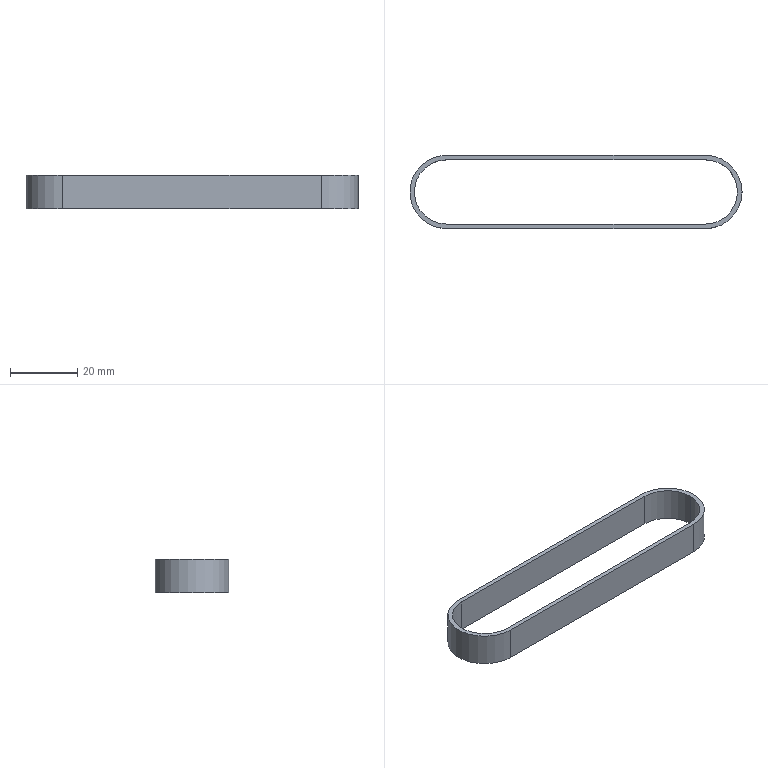Part | SolidWorks | features BaseBody 1 | 1 solid | 12 faces | box 98.817 x 21.817 x 10 mm | volume 2968 mm3 | cylinder 6 | plane 6 | commonest cylinder face diameters 19.097 x3 21.817 x3
STEP:
#1=CARTESIAN_POINT('',(45.526,9.549,0.));
#2=VERTEX_POINT('',#1);
#3=CARTESIAN_POINT('',(55.074,0.,0.));
#4=VERTEX_POINT('',#3);
#5=CARTESIAN_POINT('',(45.526,0.,0.));
#6=DIRECTION('',(0.,0.,-1.));
#7=DIRECTION('',(1.,0.,0.));
#8=AXIS2_PLACEMENT_3D('',#5,#6,#7);
#9=CIRCLE('',#8,9.549);
#10=EDGE_CURVE('',#2,#4,#9,.T.);
#11=ORIENTED_EDGE('',*,*,#10,.T.);
#12=CARTESIAN_POINT('',(55.074,0.,10.));
#13=VERTEX_POINT('',#12);
#14=CARTESIAN_POINT('',(55.074,0.,0.));
#15=DIRECTION('',(0.,0.,1.));
#16=VECTOR('',#15,1000.);
#17=LINE('',#14,#16);
#18=EDGE_CURVE('',#4,#13,#17,.T.);
#19=ORIENTED_EDGE('',*,*,#18,.T.);
#20=CARTESIAN_POINT('',(45.526,9.549,10.));
#21=VERTEX_POINT('',#20);
#22=CARTESIAN_POINT('',(45.526,0.,10.));
#23=DIRECTION('',(0.,0.,-1.));
#24=DIRECTION('',(1.,0.,0.));
#25=AXIS2_PLACEMENT_3D('',#22,#23,#24);
#26=CIRCLE('',#25,9.549);
#27=EDGE_CURVE('',#21,#13,#26,.T.);
#28=ORIENTED_EDGE('',*,*,#27,.F.);
#29=CARTESIAN_POINT('',(45.526,9.549,0.));
#30=DIRECTION('',(0.,0.,-1.));
#31=VECTOR('',#30,1000.);
#32=LINE('',#29,#31);
#33=EDGE_CURVE('',#21,#2,#32,.T.);
#34=ORIENTED_EDGE('',*,*,#33,.T.);
#35=EDGE_LOOP('',(#11,#19,#28,#34));
#36=FACE_OUTER_BOUND('',#35,.T.);
#37=CARTESIAN_POINT('',(45.526,0.,0.));
#38=DIRECTION('',(0.,0.,1.));
#39=DIRECTION('',(1.,0.,0.));
#40=AXIS2_PLACEMENT_3D('',#37,#38,#39);
#41=CYLINDRICAL_SURFACE('',#40,9.549);
#42=ADVANCED_FACE('',(#36),#41,.F.);
#43=CARTESIAN_POINT('',(45.526,-10.908,0.));
#44=VERTEX_POINT('',#43);
#45=CARTESIAN_POINT('',(56.434,0.,0.));
#46=VERTEX_POINT('',#45);
#47=CARTESIAN_POINT('',(45.526,0.,0.));
#48=DIRECTION('',(0.,0.,1.));
#49=DIRECTION('',(1.,0.,0.));
#50=AXIS2_PLACEMENT_3D('',#47,#48,#49);
#51=CIRCLE('',#50,10.909);
#52=EDGE_CURVE('',#44,#46,#51,.T.);
#53=ORIENTED_EDGE('',*,*,#52,.T.);
#54=CARTESIAN_POINT('',(56.434,0.,10.));
#55=VERTEX_POINT('',#54);
#56=CARTESIAN_POINT('',(56.434,0.,0.));
#57=DIRECTION('',(0.,0.,1.));
#58=VECTOR('',#57,1000.);
#59=LINE('',#56,#58);
#60=EDGE_CURVE('',#46,#55,#59,.T.);
#61=ORIENTED_EDGE('',*,*,#60,.T.);
#62=CARTESIAN_POINT('',(45.526,-10.908,10.));
#63=VERTEX_POINT('',#62);
#64=CARTESIAN_POINT('',(45.526,0.,10.));
#65=DIRECTION('',(0.,0.,1.));
#66=DIRECTION('',(1.,0.,0.));
#67=AXIS2_PLACEMENT_3D('',#64,#65,#66);
#68=CIRCLE('',#67,10.909);
#69=EDGE_CURVE('',#63,#55,#68,.T.);
#70=ORIENTED_EDGE('',*,*,#69,.F.);
#71=CARTESIAN_POINT('',(45.526,-10.908,0.));
#72=DIRECTION('',(0.,0.,1.));
#73=VECTOR('',#72,1000.);
#74=LINE('',#71,#73);
#75=EDGE_CURVE('',#44,#63,#74,.T.);
#76=ORIENTED_EDGE('',*,*,#75,.F.);
#77=EDGE_LOOP('',(#53,#61,#70,#76));
#78=FACE_OUTER_BOUND('',#77,.T.);
#79=CARTESIAN_POINT('',(45.526,0.,0.));
#80=DIRECTION('',(0.,0.,1.));
#81=DIRECTION('',(1.,0.,0.));
#82=AXIS2_PLACEMENT_3D('',#79,#80,#81);
#83=CYLINDRICAL_SURFACE('',#82,10.909);
#84=ADVANCED_FACE('',(#78),#83,.T.);
#85=CARTESIAN_POINT('',(-31.474,9.549,0.));
#86=VERTEX_POINT('',#85);
#87=CARTESIAN_POINT('',(-31.474,9.549,10.));
#88=VERTEX_POINT('',#87);
#89=CARTESIAN_POINT('',(-31.474,9.549,0.));
#90=DIRECTION('',(0.,0.,1.));
#91=VECTOR('',#90,1000.);
#92=LINE('',#89,#91);
#93=EDGE_CURVE('',#86,#88,#92,.T.);
#94=ORIENTED_EDGE('',*,*,#93,.F.);
#95=CARTESIAN_POINT('',(-31.474,9.549,0.));
#96=DIRECTION('',(-1.,0.,0.));
#97=VECTOR('',#96,1000.);
#98=LINE('',#95,#97);
#99=EDGE_CURVE('',#2,#86,#98,.T.);
#100=ORIENTED_EDGE('',*,*,#99,.F.);
#101=ORIENTED_EDGE('',*,*,#33,.F.);
#102=CARTESIAN_POINT('',(-31.474,9.549,10.));
#103=DIRECTION('',(1.,0.,0.));
#104=VECTOR('',#103,1000.);
#105=LINE('',#102,#104);
#106=EDGE_CURVE('',#88,#21,#105,.T.);
#107=ORIENTED_EDGE('',*,*,#106,.F.);
#108=EDGE_LOOP('',(#94,#100,#101,#107));
#109=FACE_OUTER_BOUND('',#108,.T.);
#110=CARTESIAN_POINT('',(-31.474,9.549,0.));
#111=DIRECTION('',(0.,1.,0.));
#112=DIRECTION('',(0.,0.,1.));
#113=AXIS2_PLACEMENT_3D('',#110,#111,#112);
#114=PLANE('',#113);
#115=ADVANCED_FACE('',(#109),#114,.F.);
#116=CARTESIAN_POINT('',(45.526,-9.549,10.));
#117=VERTEX_POINT('',#116);
#118=CARTESIAN_POINT('',(-31.474,-9.549,10.));
#119=VERTEX_POINT('',#118);
#120=CARTESIAN_POINT('',(7.026,-9.549,10.));
#121=DIRECTION('',(-1.,0.,0.));
#122=VECTOR('',#121,1000.);
#123=LINE('',#120,#122);
#124=EDGE_CURVE('',#117,#119,#123,.T.);
#125=ORIENTED_EDGE('',*,*,#124,.T.);
#126=CARTESIAN_POINT('',(-31.474,0.,10.));
#127=DIRECTION('',(0.,0.,-1.));
#128=DIRECTION('',(1.,0.,0.));
#129=AXIS2_PLACEMENT_3D('',#126,#127,#128);
#130=CIRCLE('',#129,9.549);
#131=EDGE_CURVE('',#119,#88,#130,.T.);
#132=ORIENTED_EDGE('',*,*,#131,.T.);
#133=ORIENTED_EDGE('',*,*,#106,.T.);
#134=ORIENTED_EDGE('',*,*,#27,.T.);
#135=CARTESIAN_POINT('',(45.526,0.,10.));
#136=DIRECTION('',(0.,0.,-1.));
#137=DIRECTION('',(1.,0.,0.));
#138=AXIS2_PLACEMENT_3D('',#135,#136,#137);
#139=CIRCLE('',#138,9.549);
#140=EDGE_CURVE('',#13,#117,#139,.T.);
#141=ORIENTED_EDGE('',*,*,#140,.T.);
#142=EDGE_LOOP('',(#125,#132,#133,#134,#141));
#143=FACE_BOUND('',#142,.T.);
#144=CARTESIAN_POINT('',(-31.474,10.908,10.));
#145=VERTEX_POINT('',#144);
#146=CARTESIAN_POINT('',(-31.474,-10.908,10.));
#147=VERTEX_POINT('',#146);
#148=CARTESIAN_POINT('',(-31.474,0.,10.));
#149=DIRECTION('',(0.,0.,1.));
#150=DIRECTION('',(1.,0.,0.));
#151=AXIS2_PLACEMENT_3D('',#148,#149,#150);
#152=CIRCLE('',#151,10.909);
#153=EDGE_CURVE('',#145,#147,#152,.T.);
#154=ORIENTED_EDGE('',*,*,#153,.T.);
#155=CARTESIAN_POINT('',(7.026,-10.908,10.));
#156=DIRECTION('',(1.,0.,0.));
#157=VECTOR('',#156,1000.);
#158=LINE('',#155,#157);
#159=EDGE_CURVE('',#147,#63,#158,.T.);
#160=ORIENTED_EDGE('',*,*,#159,.T.);
#161=ORIENTED_EDGE('',*,*,#69,.T.);
#162=CARTESIAN_POINT('',(45.526,10.908,10.));
#163=VERTEX_POINT('',#162);
#164=CARTESIAN_POINT('',(45.526,0.,10.));
#165=DIRECTION('',(0.,0.,1.));
#166=DIRECTION('',(1.,0.,0.));
#167=AXIS2_PLACEMENT_3D('',#164,#165,#166);
#168=CIRCLE('',#167,10.909);
#169=EDGE_CURVE('',#55,#163,#168,.T.);
#170=ORIENTED_EDGE('',*,*,#169,.T.);
#171=CARTESIAN_POINT('',(7.026,10.908,10.));
#172=DIRECTION('',(-1.,0.,0.));
#173=VECTOR('',#172,1000.);
#174=LINE('',#171,#173);
#175=EDGE_CURVE('',#163,#145,#174,.T.);
#176=ORIENTED_EDGE('',*,*,#175,.T.);
#177=EDGE_LOOP('',(#154,#160,#161,#170,#176));
#178=FACE_OUTER_BOUND('',#177,.T.);
#179=CARTESIAN_POINT('',(7.026,0.,10.));
#180=DIRECTION('',(0.,0.,1.));
#181=DIRECTION('',(1.,0.,0.));
#182=AXIS2_PLACEMENT_3D('',#179,#180,#181);
#183=PLANE('',#182);
#184=ADVANCED_FACE('',(#143,#178),#183,.T.);
#185=CARTESIAN_POINT('',(-31.474,-9.549,0.));
#186=VERTEX_POINT('',#185);
#187=CARTESIAN_POINT('',(-31.474,-9.549,0.));
#188=DIRECTION('',(0.,0.,1.));
#189=VECTOR('',#188,1000.);
#190=LINE('',#187,#189);
#191=EDGE_CURVE('',#186,#119,#190,.T.);
#192=ORIENTED_EDGE('',*,*,#191,.F.);
#193=CARTESIAN_POINT('',(-31.474,0.,0.));
#194=DIRECTION('',(0.,0.,1.));
#195=DIRECTION('',(1.,0.,0.));
#196=AXIS2_PLACEMENT_3D('',#193,#194,#195);
#197=CIRCLE('',#196,9.549);
#198=EDGE_CURVE('',#86,#186,#197,.T.);
#199=ORIENTED_EDGE('',*,*,#198,.F.);
#200=ORIENTED_EDGE('',*,*,#93,.T.);
#201=ORIENTED_EDGE('',*,*,#131,.F.);
#202=EDGE_LOOP('',(#192,#199,#200,#201));
#203=FACE_OUTER_BOUND('',#202,.T.);
#204=CARTESIAN_POINT('',(-31.474,0.,0.));
#205=DIRECTION('',(0.,0.,1.));
#206=DIRECTION('',(1.,0.,0.));
#207=AXIS2_PLACEMENT_3D('',#204,#205,#206);
#208=CYLINDRICAL_SURFACE('',#207,9.549);
#209=ADVANCED_FACE('',(#203),#208,.F.);
#210=ORIENTED_EDGE('',*,*,#198,.T.);
#211=CARTESIAN_POINT('',(45.526,-9.549,0.));
#212=VERTEX_POINT('',#211);
#213=CARTESIAN_POINT('',(7.026,-9.549,0.));
#214=DIRECTION('',(-1.,0.,0.));
#215=VECTOR('',#214,1000.);
#216=LINE('',#213,#215);
#217=EDGE_CURVE('',#212,#186,#216,.T.);
#218=ORIENTED_EDGE('',*,*,#217,.F.);
#219=CARTESIAN_POINT('',(45.526,0.,0.));
#220=DIRECTION('',(0.,0.,-1.));
#221=DIRECTION('',(1.,0.,0.));
#222=AXIS2_PLACEMENT_3D('',#219,#220,#221);
#223=CIRCLE('',#222,9.549);
#224=EDGE_CURVE('',#4,#212,#223,.T.);
#225=ORIENTED_EDGE('',*,*,#224,.F.);
#226=ORIENTED_EDGE('',*,*,#10,.F.);
#227=ORIENTED_EDGE('',*,*,#99,.T.);
#228=EDGE_LOOP('',(#210,#218,#225,#226,#227));
#229=FACE_BOUND('',#228,.T.);
#230=ORIENTED_EDGE('',*,*,#52,.F.);
#231=CARTESIAN_POINT('',(-31.474,-10.908,0.));
#232=VERTEX_POINT('',#231);
#233=CARTESIAN_POINT('',(7.026,-10.908,0.));
#234=DIRECTION('',(1.,0.,0.));
#235=VECTOR('',#234,1000.);
#236=LINE('',#233,#235);
#237=EDGE_CURVE('',#232,#44,#236,.T.);
#238=ORIENTED_EDGE('',*,*,#237,.F.);
#239=CARTESIAN_POINT('',(-31.474,10.908,0.));
#240=VERTEX_POINT('',#239);
#241=CARTESIAN_POINT('',(-31.474,0.,0.));
#242=DIRECTION('',(0.,0.,1.));
#243=DIRECTION('',(1.,0.,0.));
#244=AXIS2_PLACEMENT_3D('',#241,#242,#243);
#245=CIRCLE('',#244,10.909);
#246=EDGE_CURVE('',#240,#232,#245,.T.);
#247=ORIENTED_EDGE('',*,*,#246,.F.);
#248=CARTESIAN_POINT('',(45.526,10.908,0.));
#249=VERTEX_POINT('',#248);
#250=CARTESIAN_POINT('',(7.026,10.908,0.));
#251=DIRECTION('',(-1.,0.,0.));
#252=VECTOR('',#251,1000.);
#253=LINE('',#250,#252);
#254=EDGE_CURVE('',#249,#240,#253,.T.);
#255=ORIENTED_EDGE('',*,*,#254,.F.);
#256=CARTESIAN_POINT('',(45.526,0.,0.));
#257=DIRECTION('',(0.,0.,1.));
#258=DIRECTION('',(1.,0.,0.));
#259=AXIS2_PLACEMENT_3D('',#256,#257,#258);
#260=CIRCLE('',#259,10.909);
#261=EDGE_CURVE('',#46,#249,#260,.T.);
#262=ORIENTED_EDGE('',*,*,#261,.F.);
#263=EDGE_LOOP('',(#230,#238,#247,#255,#262));
#264=FACE_OUTER_BOUND('',#263,.T.);
#265=CARTESIAN_POINT('',(7.026,0.,0.));
#266=DIRECTION('',(0.,0.,1.));
#267=DIRECTION('',(1.,0.,0.));
#268=AXIS2_PLACEMENT_3D('',#265,#266,#267);
#269=PLANE('',#268);
#270=ADVANCED_FACE('',(#229,#264),#269,.F.);
#271=ORIENTED_EDGE('',*,*,#18,.F.);
#272=ORIENTED_EDGE('',*,*,#224,.T.);
#273=CARTESIAN_POINT('',(45.526,-9.549,0.));
#274=DIRECTION('',(0.,0.,-1.));
#275=VECTOR('',#274,1000.);
#276=LINE('',#273,#275);
#277=EDGE_CURVE('',#117,#212,#276,.T.);
#278=ORIENTED_EDGE('',*,*,#277,.F.);
#279=ORIENTED_EDGE('',*,*,#140,.F.);
#280=EDGE_LOOP('',(#271,#272,#278,#279));
#281=FACE_OUTER_BOUND('',#280,.T.);
#282=CARTESIAN_POINT('',(45.526,0.,0.));
#283=DIRECTION('',(0.,0.,1.));
#284=DIRECTION('',(1.,0.,0.));
#285=AXIS2_PLACEMENT_3D('',#282,#283,#284);
#286=CYLINDRICAL_SURFACE('',#285,9.549);
#287=ADVANCED_FACE('',(#281),#286,.F.);
#288=ORIENTED_EDGE('',*,*,#277,.T.);
#289=ORIENTED_EDGE('',*,*,#217,.T.);
#290=ORIENTED_EDGE('',*,*,#191,.T.);
#291=ORIENTED_EDGE('',*,*,#124,.F.);
#292=EDGE_LOOP('',(#288,#289,#290,#291));
#293=FACE_OUTER_BOUND('',#292,.T.);
#294=CARTESIAN_POINT('',(45.526,-9.549,0.));
#295=DIRECTION('',(0.,-1.,0.));
#296=DIRECTION('',(0.,0.,-1.));
#297=AXIS2_PLACEMENT_3D('',#294,#295,#296);
#298=PLANE('',#297);
#299=ADVANCED_FACE('',(#293),#298,.F.);
#300=ORIENTED_EDGE('',*,*,#237,.T.);
#301=ORIENTED_EDGE('',*,*,#75,.T.);
#302=ORIENTED_EDGE('',*,*,#159,.F.);
#303=CARTESIAN_POINT('',(-31.474,-10.908,0.));
#304=DIRECTION('',(0.,0.,-1.));
#305=VECTOR('',#304,1000.);
#306=LINE('',#303,#305);
#307=EDGE_CURVE('',#147,#232,#306,.T.);
#308=ORIENTED_EDGE('',*,*,#307,.T.);
#309=EDGE_LOOP('',(#300,#301,#302,#308));
#310=FACE_OUTER_BOUND('',#309,.T.);
#311=CARTESIAN_POINT('',(45.526,-10.908,0.));
#312=DIRECTION('',(0.,-1.,0.));
#313=DIRECTION('',(0.,0.,-1.));
#314=AXIS2_PLACEMENT_3D('',#311,#312,#313);
#315=PLANE('',#314);
#316=ADVANCED_FACE('',(#310),#315,.T.);
#317=ORIENTED_EDGE('',*,*,#246,.T.);
#318=ORIENTED_EDGE('',*,*,#307,.F.);
#319=ORIENTED_EDGE('',*,*,#153,.F.);
#320=CARTESIAN_POINT('',(-31.474,10.909,0.));
#321=DIRECTION('',(0.,0.,-1.));
#322=VECTOR('',#321,1000.);
#323=LINE('',#320,#322);
#324=EDGE_CURVE('',#145,#240,#323,.T.);
#325=ORIENTED_EDGE('',*,*,#324,.T.);
#326=EDGE_LOOP('',(#317,#318,#319,#325));
#327=FACE_OUTER_BOUND('',#326,.T.);
#328=CARTESIAN_POINT('',(-31.474,0.,0.));
#329=DIRECTION('',(0.,0.,1.));
#330=DIRECTION('',(1.,0.,0.));
#331=AXIS2_PLACEMENT_3D('',#328,#329,#330);
#332=CYLINDRICAL_SURFACE('',#331,10.909);
#333=ADVANCED_FACE('',(#327),#332,.T.);
#334=ORIENTED_EDGE('',*,*,#254,.T.);
#335=ORIENTED_EDGE('',*,*,#324,.F.);
#336=ORIENTED_EDGE('',*,*,#175,.F.);
#337=CARTESIAN_POINT('',(45.526,10.908,0.));
#338=DIRECTION('',(0.,0.,-1.));
#339=VECTOR('',#338,1000.);
#340=LINE('',#337,#339);
#341=EDGE_CURVE('',#163,#249,#340,.T.);
#342=ORIENTED_EDGE('',*,*,#341,.T.);
#343=EDGE_LOOP('',(#334,#335,#336,#342));
#344=FACE_OUTER_BOUND('',#343,.T.);
#345=CARTESIAN_POINT('',(-31.474,10.908,0.));
#346=DIRECTION('',(0.,1.,0.));
#347=DIRECTION('',(0.,0.,1.));
#348=AXIS2_PLACEMENT_3D('',#345,#346,#347);
#349=PLANE('',#348);
#350=ADVANCED_FACE('',(#344),#349,.T.);
#351=ORIENTED_EDGE('',*,*,#60,.F.);
#352=ORIENTED_EDGE('',*,*,#261,.T.);
#353=ORIENTED_EDGE('',*,*,#341,.F.);
#354=ORIENTED_EDGE('',*,*,#169,.F.);
#355=EDGE_LOOP('',(#351,#352,#353,#354));
#356=FACE_OUTER_BOUND('',#355,.T.);
#357=CARTESIAN_POINT('',(45.526,0.,0.));
#358=DIRECTION('',(0.,0.,1.));
#359=DIRECTION('',(1.,0.,0.));
#360=AXIS2_PLACEMENT_3D('',#357,#358,#359);
#361=CYLINDRICAL_SURFACE('',#360,10.909);
#362=ADVANCED_FACE('',(#356),#361,.T.);
#363=CLOSED_SHELL('',(#42,#84,#115,#184,#209,#270,#287,#299,#316,#333,#350,#362));
#364=MANIFOLD_SOLID_BREP('',#363);
#365=CARTESIAN_POINT('',(0.,0.,0.));
#366=DIRECTION('',(0.,0.,1.));
#367=DIRECTION('',(1.,0.,0.));
#368=AXIS2_PLACEMENT_3D('',#365,#366,#367);
#369=(LENGTH_UNIT()NAMED_UNIT(*)SI_UNIT(.MILLI.,.METRE.));
#370=UNCERTAINTY_MEASURE_WITH_UNIT(LENGTH_MEASURE(0.00001),#369,'','');
#371=(NAMED_UNIT(*)PLANE_ANGLE_UNIT()SI_UNIT($,.RADIAN.));
#372=(NAMED_UNIT(*)SI_UNIT($,.STERADIAN.)SOLID_ANGLE_UNIT());
#373=(GEOMETRIC_REPRESENTATION_CONTEXT(3)GLOBAL_UNCERTAINTY_ASSIGNED_CONTEXT((#370))GLOBAL_UNIT_ASSIGNED_CONTEXT((#369,#371,#372))REPRESENTATION_CONTEXT('',''));
#374=ADVANCED_BREP_SHAPE_REPRESENTATION('',(#364,#368),#373);